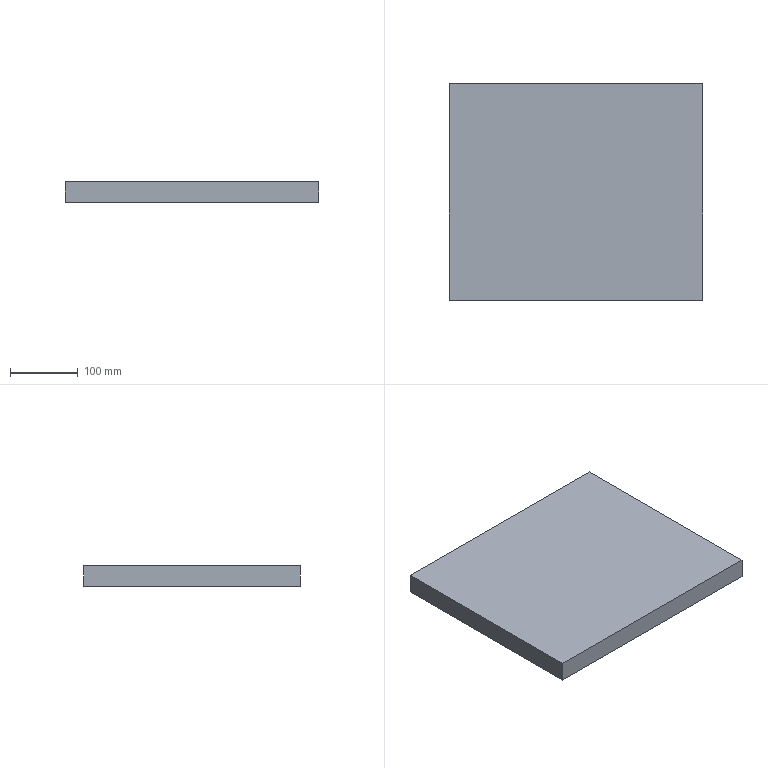Part | STEP file | PN_0008 Pump body base plate | 1 solid | 6 faces | box 375 x 320 x 30 mm | volume 3600000 mm3 | plane 6
STEP:
#1=CARTESIAN_POINT('',(0.,0.,0.));
#2=DIRECTION('',(0.,0.,1.));
#3=DIRECTION('',(1.,0.,0.));
#4=AXIS2_PLACEMENT_3D('',#1,#2,#3);
#5=CARTESIAN_POINT('',(0.,0.,0.));
#6=VERTEX_POINT('',#5);
#7=CARTESIAN_POINT('',(0.,0.,30.));
#8=VERTEX_POINT('',#7);
#9=CARTESIAN_POINT('',(0.,0.,0.));
#10=DIRECTION('',(0.,0.,1.));
#11=VECTOR('',#10,1.);
#12=LINE('',#9,#11);
#13=CARTESIAN_POINT('',(0.,320.,0.));
#14=DIRECTION('',(1.,0.,0.));
#15=DIRECTION('',(0.,0.,-1.));
#16=AXIS2_PLACEMENT_3D('',#13,#14,#15);
#17=PLANE('',#16);
#18=CARTESIAN_POINT('',(0.,-320.));
#19=DIRECTION('',(-1.,0.));
#20=VECTOR('',#19,1.);
#21=LINE('',#18,#20);
#22=(GEOMETRIC_REPRESENTATION_CONTEXT(2)PARAMETRIC_REPRESENTATION_CONTEXT()REPRESENTATION_CONTEXT('',''));
#23=DEFINITIONAL_REPRESENTATION('',(#21),#22);
#24=PCURVE('',#17,#23);
#25=CARTESIAN_POINT('',(0.,0.,30.));
#26=DIRECTION('',(0.,1.,0.));
#27=DIRECTION('',(0.,0.,1.));
#28=AXIS2_PLACEMENT_3D('',#25,#26,#27);
#29=PLANE('',#28);
#30=CARTESIAN_POINT('',(-30.,0.));
#31=DIRECTION('',(1.,0.));
#32=VECTOR('',#31,1.);
#33=LINE('',#30,#32);
#34=(GEOMETRIC_REPRESENTATION_CONTEXT(2)PARAMETRIC_REPRESENTATION_CONTEXT()REPRESENTATION_CONTEXT('',''));
#35=DEFINITIONAL_REPRESENTATION('',(#33),#34);
#36=PCURVE('',#29,#35);
#37=SURFACE_CURVE('',#12,(#24,#36),.PCURVE_S1.);
#38=EDGE_CURVE('',#6,#8,#37,.T.);
#39=ORIENTED_EDGE('',*,*,#38,.T.);
#40=CARTESIAN_POINT('',(0.,320.,30.));
#41=VERTEX_POINT('',#40);
#42=CARTESIAN_POINT('',(0.,320.,30.));
#43=DIRECTION('',(0.,-1.,0.));
#44=VECTOR('',#43,1.);
#45=LINE('',#42,#44);
#46=CARTESIAN_POINT('',(-30.,0.));
#47=DIRECTION('',(0.,-1.));
#48=VECTOR('',#47,1.);
#49=LINE('',#46,#48);
#50=(GEOMETRIC_REPRESENTATION_CONTEXT(2)PARAMETRIC_REPRESENTATION_CONTEXT()REPRESENTATION_CONTEXT('',''));
#51=DEFINITIONAL_REPRESENTATION('',(#49),#50);
#52=PCURVE('',#17,#51);
#53=CARTESIAN_POINT('',(0.,320.,30.));
#54=DIRECTION('',(0.,0.,-1.));
#55=DIRECTION('',(-1.,0.,0.));
#56=AXIS2_PLACEMENT_3D('',#53,#54,#55);
#57=PLANE('',#56);
#58=CARTESIAN_POINT('',(0.,0.));
#59=DIRECTION('',(0.,-1.));
#60=VECTOR('',#59,1.);
#61=LINE('',#58,#60);
#62=(GEOMETRIC_REPRESENTATION_CONTEXT(2)PARAMETRIC_REPRESENTATION_CONTEXT()REPRESENTATION_CONTEXT('',''));
#63=DEFINITIONAL_REPRESENTATION('',(#61),#62);
#64=PCURVE('',#57,#63);
#65=SURFACE_CURVE('',#45,(#52,#64),.PCURVE_S1.);
#66=EDGE_CURVE('',#41,#8,#65,.T.);
#67=ORIENTED_EDGE('',*,*,#66,.F.);
#68=CARTESIAN_POINT('',(0.,320.,0.));
#69=VERTEX_POINT('',#68);
#70=CARTESIAN_POINT('',(0.,320.,0.));
#71=DIRECTION('',(0.,0.,1.));
#72=VECTOR('',#71,1.);
#73=LINE('',#70,#72);
#74=CARTESIAN_POINT('',(0.,0.));
#75=DIRECTION('',(-1.,0.));
#76=VECTOR('',#75,1.);
#77=LINE('',#74,#76);
#78=(GEOMETRIC_REPRESENTATION_CONTEXT(2)PARAMETRIC_REPRESENTATION_CONTEXT()REPRESENTATION_CONTEXT('',''));
#79=DEFINITIONAL_REPRESENTATION('',(#77),#78);
#80=PCURVE('',#17,#79);
#81=CARTESIAN_POINT('',(0.,320.,30.));
#82=DIRECTION('',(0.,1.,0.));
#83=DIRECTION('',(0.,0.,1.));
#84=AXIS2_PLACEMENT_3D('',#81,#82,#83);
#85=PLANE('',#84);
#86=CARTESIAN_POINT('',(-30.,0.));
#87=DIRECTION('',(1.,0.));
#88=VECTOR('',#87,1.);
#89=LINE('',#86,#88);
#90=(GEOMETRIC_REPRESENTATION_CONTEXT(2)PARAMETRIC_REPRESENTATION_CONTEXT()REPRESENTATION_CONTEXT('',''));
#91=DEFINITIONAL_REPRESENTATION('',(#89),#90);
#92=PCURVE('',#85,#91);
#93=SURFACE_CURVE('',#73,(#80,#92),.PCURVE_S1.);
#94=EDGE_CURVE('',#69,#41,#93,.T.);
#95=ORIENTED_EDGE('',*,*,#94,.F.);
#96=CARTESIAN_POINT('',(0.,320.,0.));
#97=DIRECTION('',(0.,-1.,0.));
#98=VECTOR('',#97,1.);
#99=LINE('',#96,#98);
#100=CARTESIAN_POINT('',(0.,0.));
#101=DIRECTION('',(0.,-1.));
#102=VECTOR('',#101,1.);
#103=LINE('',#100,#102);
#104=(GEOMETRIC_REPRESENTATION_CONTEXT(2)PARAMETRIC_REPRESENTATION_CONTEXT()REPRESENTATION_CONTEXT('',''));
#105=DEFINITIONAL_REPRESENTATION('',(#103),#104);
#106=PCURVE('',#17,#105);
#107=CARTESIAN_POINT('',(0.,320.,0.));
#108=DIRECTION('',(0.,0.,1.));
#109=DIRECTION('',(1.,0.,0.));
#110=AXIS2_PLACEMENT_3D('',#107,#108,#109);
#111=PLANE('',#110);
#112=CARTESIAN_POINT('',(0.,0.));
#113=DIRECTION('',(0.,-1.));
#114=VECTOR('',#113,1.);
#115=LINE('',#112,#114);
#116=(GEOMETRIC_REPRESENTATION_CONTEXT(2)PARAMETRIC_REPRESENTATION_CONTEXT()REPRESENTATION_CONTEXT('',''));
#117=DEFINITIONAL_REPRESENTATION('',(#115),#116);
#118=PCURVE('',#111,#117);
#119=SURFACE_CURVE('',#99,(#106,#118),.PCURVE_S1.);
#120=EDGE_CURVE('',#69,#6,#119,.T.);
#121=ORIENTED_EDGE('',*,*,#120,.T.);
#122=EDGE_LOOP('',(#39,#67,#95,#121));
#123=FACE_BOUND('',#122,.T.);
#124=ADVANCED_FACE('',(#123),#17,.F.);
#125=CARTESIAN_POINT('',(375.,0.,30.));
#126=VERTEX_POINT('',#125);
#127=CARTESIAN_POINT('',(0.,0.,30.));
#128=DIRECTION('',(1.,0.,0.));
#129=VECTOR('',#128,1.);
#130=LINE('',#127,#129);
#131=CARTESIAN_POINT('',(0.,-320.));
#132=DIRECTION('',(-1.,0.));
#133=VECTOR('',#132,1.);
#134=LINE('',#131,#133);
#135=(GEOMETRIC_REPRESENTATION_CONTEXT(2)PARAMETRIC_REPRESENTATION_CONTEXT()REPRESENTATION_CONTEXT('',''));
#136=DEFINITIONAL_REPRESENTATION('',(#134),#135);
#137=PCURVE('',#57,#136);
#138=CARTESIAN_POINT('',(0.,0.));
#139=DIRECTION('',(0.,1.));
#140=VECTOR('',#139,1.);
#141=LINE('',#138,#140);
#142=(GEOMETRIC_REPRESENTATION_CONTEXT(2)PARAMETRIC_REPRESENTATION_CONTEXT()REPRESENTATION_CONTEXT('',''));
#143=DEFINITIONAL_REPRESENTATION('',(#141),#142);
#144=PCURVE('',#29,#143);
#145=SURFACE_CURVE('',#130,(#137,#144),.PCURVE_S1.);
#146=EDGE_CURVE('',#8,#126,#145,.T.);
#147=ORIENTED_EDGE('',*,*,#146,.T.);
#148=CARTESIAN_POINT('',(375.,320.,30.));
#149=VERTEX_POINT('',#148);
#150=CARTESIAN_POINT('',(375.,320.,30.));
#151=DIRECTION('',(0.,-1.,0.));
#152=VECTOR('',#151,1.);
#153=LINE('',#150,#152);
#154=CARTESIAN_POINT('',(-375.,0.));
#155=DIRECTION('',(0.,-1.));
#156=VECTOR('',#155,1.);
#157=LINE('',#154,#156);
#158=(GEOMETRIC_REPRESENTATION_CONTEXT(2)PARAMETRIC_REPRESENTATION_CONTEXT()REPRESENTATION_CONTEXT('',''));
#159=DEFINITIONAL_REPRESENTATION('',(#157),#158);
#160=PCURVE('',#57,#159);
#161=CARTESIAN_POINT('',(375.,320.,0.));
#162=DIRECTION('',(-1.,0.,0.));
#163=DIRECTION('',(0.,0.,1.));
#164=AXIS2_PLACEMENT_3D('',#161,#162,#163);
#165=PLANE('',#164);
#166=CARTESIAN_POINT('',(30.,0.));
#167=DIRECTION('',(0.,-1.));
#168=VECTOR('',#167,1.);
#169=LINE('',#166,#168);
#170=(GEOMETRIC_REPRESENTATION_CONTEXT(2)PARAMETRIC_REPRESENTATION_CONTEXT()REPRESENTATION_CONTEXT('',''));
#171=DEFINITIONAL_REPRESENTATION('',(#169),#170);
#172=PCURVE('',#165,#171);
#173=SURFACE_CURVE('',#153,(#160,#172),.PCURVE_S1.);
#174=EDGE_CURVE('',#149,#126,#173,.T.);
#175=ORIENTED_EDGE('',*,*,#174,.F.);
#176=CARTESIAN_POINT('',(0.,320.,30.));
#177=DIRECTION('',(1.,0.,0.));
#178=VECTOR('',#177,1.);
#179=LINE('',#176,#178);
#180=CARTESIAN_POINT('',(0.,0.));
#181=DIRECTION('',(-1.,0.));
#182=VECTOR('',#181,1.);
#183=LINE('',#180,#182);
#184=(GEOMETRIC_REPRESENTATION_CONTEXT(2)PARAMETRIC_REPRESENTATION_CONTEXT()REPRESENTATION_CONTEXT('',''));
#185=DEFINITIONAL_REPRESENTATION('',(#183),#184);
#186=PCURVE('',#57,#185);
#187=CARTESIAN_POINT('',(0.,0.));
#188=DIRECTION('',(0.,1.));
#189=VECTOR('',#188,1.);
#190=LINE('',#187,#189);
#191=(GEOMETRIC_REPRESENTATION_CONTEXT(2)PARAMETRIC_REPRESENTATION_CONTEXT()REPRESENTATION_CONTEXT('',''));
#192=DEFINITIONAL_REPRESENTATION('',(#190),#191);
#193=PCURVE('',#85,#192);
#194=SURFACE_CURVE('',#179,(#186,#193),.PCURVE_S1.);
#195=EDGE_CURVE('',#41,#149,#194,.T.);
#196=ORIENTED_EDGE('',*,*,#195,.F.);
#197=ORIENTED_EDGE('',*,*,#66,.T.);
#198=EDGE_LOOP('',(#147,#175,#196,#197));
#199=FACE_BOUND('',#198,.T.);
#200=ADVANCED_FACE('',(#199),#57,.F.);
#201=CARTESIAN_POINT('',(375.,0.,0.));
#202=VERTEX_POINT('',#201);
#203=CARTESIAN_POINT('',(375.,0.,0.));
#204=DIRECTION('',(0.,0.,-1.));
#205=VECTOR('',#204,1.);
#206=LINE('',#203,#205);
#207=CARTESIAN_POINT('',(0.,-320.));
#208=DIRECTION('',(-1.,0.));
#209=VECTOR('',#208,1.);
#210=LINE('',#207,#209);
#211=(GEOMETRIC_REPRESENTATION_CONTEXT(2)PARAMETRIC_REPRESENTATION_CONTEXT()REPRESENTATION_CONTEXT('',''));
#212=DEFINITIONAL_REPRESENTATION('',(#210),#211);
#213=PCURVE('',#165,#212);
#214=CARTESIAN_POINT('',(-30.,375.));
#215=DIRECTION('',(-1.,0.));
#216=VECTOR('',#215,1.);
#217=LINE('',#214,#216);
#218=(GEOMETRIC_REPRESENTATION_CONTEXT(2)PARAMETRIC_REPRESENTATION_CONTEXT()REPRESENTATION_CONTEXT('',''));
#219=DEFINITIONAL_REPRESENTATION('',(#217),#218);
#220=PCURVE('',#29,#219);
#221=SURFACE_CURVE('',#206,(#213,#220),.PCURVE_S1.);
#222=EDGE_CURVE('',#126,#202,#221,.T.);
#223=ORIENTED_EDGE('',*,*,#222,.T.);
#224=CARTESIAN_POINT('',(375.,320.,0.));
#225=VERTEX_POINT('',#224);
#226=CARTESIAN_POINT('',(375.,320.,0.));
#227=DIRECTION('',(0.,-1.,0.));
#228=VECTOR('',#227,1.);
#229=LINE('',#226,#228);
#230=CARTESIAN_POINT('',(0.,0.));
#231=DIRECTION('',(0.,-1.));
#232=VECTOR('',#231,1.);
#233=LINE('',#230,#232);
#234=(GEOMETRIC_REPRESENTATION_CONTEXT(2)PARAMETRIC_REPRESENTATION_CONTEXT()REPRESENTATION_CONTEXT('',''));
#235=DEFINITIONAL_REPRESENTATION('',(#233),#234);
#236=PCURVE('',#165,#235);
#237=CARTESIAN_POINT('',(375.,0.));
#238=DIRECTION('',(0.,-1.));
#239=VECTOR('',#238,1.);
#240=LINE('',#237,#239);
#241=(GEOMETRIC_REPRESENTATION_CONTEXT(2)PARAMETRIC_REPRESENTATION_CONTEXT()REPRESENTATION_CONTEXT('',''));
#242=DEFINITIONAL_REPRESENTATION('',(#240),#241);
#243=PCURVE('',#111,#242);
#244=SURFACE_CURVE('',#229,(#236,#243),.PCURVE_S1.);
#245=EDGE_CURVE('',#225,#202,#244,.T.);
#246=ORIENTED_EDGE('',*,*,#245,.F.);
#247=CARTESIAN_POINT('',(375.,320.,0.));
#248=DIRECTION('',(0.,0.,-1.));
#249=VECTOR('',#248,1.);
#250=LINE('',#247,#249);
#251=CARTESIAN_POINT('',(0.,0.));
#252=DIRECTION('',(-1.,0.));
#253=VECTOR('',#252,1.);
#254=LINE('',#251,#253);
#255=(GEOMETRIC_REPRESENTATION_CONTEXT(2)PARAMETRIC_REPRESENTATION_CONTEXT()REPRESENTATION_CONTEXT('',''));
#256=DEFINITIONAL_REPRESENTATION('',(#254),#255);
#257=PCURVE('',#165,#256);
#258=CARTESIAN_POINT('',(-30.,375.));
#259=DIRECTION('',(-1.,0.));
#260=VECTOR('',#259,1.);
#261=LINE('',#258,#260);
#262=(GEOMETRIC_REPRESENTATION_CONTEXT(2)PARAMETRIC_REPRESENTATION_CONTEXT()REPRESENTATION_CONTEXT('',''));
#263=DEFINITIONAL_REPRESENTATION('',(#261),#262);
#264=PCURVE('',#85,#263);
#265=SURFACE_CURVE('',#250,(#257,#264),.PCURVE_S1.);
#266=EDGE_CURVE('',#149,#225,#265,.T.);
#267=ORIENTED_EDGE('',*,*,#266,.F.);
#268=ORIENTED_EDGE('',*,*,#174,.T.);
#269=EDGE_LOOP('',(#223,#246,#267,#268));
#270=FACE_BOUND('',#269,.T.);
#271=ADVANCED_FACE('',(#270),#165,.F.);
#272=CARTESIAN_POINT('',(0.,0.,0.));
#273=DIRECTION('',(-1.,0.,0.));
#274=VECTOR('',#273,1.);
#275=LINE('',#272,#274);
#276=CARTESIAN_POINT('',(0.,-320.));
#277=DIRECTION('',(-1.,0.));
#278=VECTOR('',#277,1.);
#279=LINE('',#276,#278);
#280=(GEOMETRIC_REPRESENTATION_CONTEXT(2)PARAMETRIC_REPRESENTATION_CONTEXT()REPRESENTATION_CONTEXT('',''));
#281=DEFINITIONAL_REPRESENTATION('',(#279),#280);
#282=PCURVE('',#111,#281);
#283=CARTESIAN_POINT('',(-30.,0.));
#284=DIRECTION('',(0.,-1.));
#285=VECTOR('',#284,1.);
#286=LINE('',#283,#285);
#287=(GEOMETRIC_REPRESENTATION_CONTEXT(2)PARAMETRIC_REPRESENTATION_CONTEXT()REPRESENTATION_CONTEXT('',''));
#288=DEFINITIONAL_REPRESENTATION('',(#286),#287);
#289=PCURVE('',#29,#288);
#290=SURFACE_CURVE('',#275,(#282,#289),.PCURVE_S1.);
#291=EDGE_CURVE('',#202,#6,#290,.T.);
#292=ORIENTED_EDGE('',*,*,#291,.T.);
#293=ORIENTED_EDGE('',*,*,#120,.F.);
#294=CARTESIAN_POINT('',(0.,320.,0.));
#295=DIRECTION('',(-1.,0.,0.));
#296=VECTOR('',#295,1.);
#297=LINE('',#294,#296);
#298=CARTESIAN_POINT('',(0.,0.));
#299=DIRECTION('',(-1.,0.));
#300=VECTOR('',#299,1.);
#301=LINE('',#298,#300);
#302=(GEOMETRIC_REPRESENTATION_CONTEXT(2)PARAMETRIC_REPRESENTATION_CONTEXT()REPRESENTATION_CONTEXT('',''));
#303=DEFINITIONAL_REPRESENTATION('',(#301),#302);
#304=PCURVE('',#111,#303);
#305=CARTESIAN_POINT('',(-30.,0.));
#306=DIRECTION('',(0.,-1.));
#307=VECTOR('',#306,1.);
#308=LINE('',#305,#307);
#309=(GEOMETRIC_REPRESENTATION_CONTEXT(2)PARAMETRIC_REPRESENTATION_CONTEXT()REPRESENTATION_CONTEXT('',''));
#310=DEFINITIONAL_REPRESENTATION('',(#308),#309);
#311=PCURVE('',#85,#310);
#312=SURFACE_CURVE('',#297,(#304,#311),.PCURVE_S1.);
#313=EDGE_CURVE('',#225,#69,#312,.T.);
#314=ORIENTED_EDGE('',*,*,#313,.F.);
#315=ORIENTED_EDGE('',*,*,#245,.T.);
#316=EDGE_LOOP('',(#292,#293,#314,#315));
#317=FACE_BOUND('',#316,.T.);
#318=ADVANCED_FACE('',(#317),#111,.F.);
#319=ORIENTED_EDGE('',*,*,#94,.T.);
#320=ORIENTED_EDGE('',*,*,#195,.T.);
#321=ORIENTED_EDGE('',*,*,#266,.T.);
#322=ORIENTED_EDGE('',*,*,#313,.T.);
#323=EDGE_LOOP('',(#319,#320,#321,#322));
#324=FACE_BOUND('',#323,.T.);
#325=ADVANCED_FACE('',(#324),#85,.T.);
#326=ORIENTED_EDGE('',*,*,#38,.F.);
#327=ORIENTED_EDGE('',*,*,#291,.F.);
#328=ORIENTED_EDGE('',*,*,#222,.F.);
#329=ORIENTED_EDGE('',*,*,#146,.F.);
#330=EDGE_LOOP('',(#326,#327,#328,#329));
#331=FACE_BOUND('',#330,.T.);
#332=ADVANCED_FACE('',(#331),#29,.F.);
#333=CLOSED_SHELL('',(#124,#200,#271,#318,#325,#332));
#334=MANIFOLD_SOLID_BREP('',#333);
#335=(LENGTH_UNIT()NAMED_UNIT(*)SI_UNIT(.MILLI.,.METRE.));
#336=UNCERTAINTY_MEASURE_WITH_UNIT(LENGTH_MEASURE(0.0000001),#335,'','');
#337=(NAMED_UNIT(*)PLANE_ANGLE_UNIT()SI_UNIT($,.RADIAN.));
#338=(NAMED_UNIT(*)SI_UNIT($,.STERADIAN.)SOLID_ANGLE_UNIT());
#339=(GEOMETRIC_REPRESENTATION_CONTEXT(3)GLOBAL_UNCERTAINTY_ASSIGNED_CONTEXT((#336))GLOBAL_UNIT_ASSIGNED_CONTEXT((#335,#337,#338))REPRESENTATION_CONTEXT('',''));
#340=ADVANCED_BREP_SHAPE_REPRESENTATION('',(#4,#334),#339);